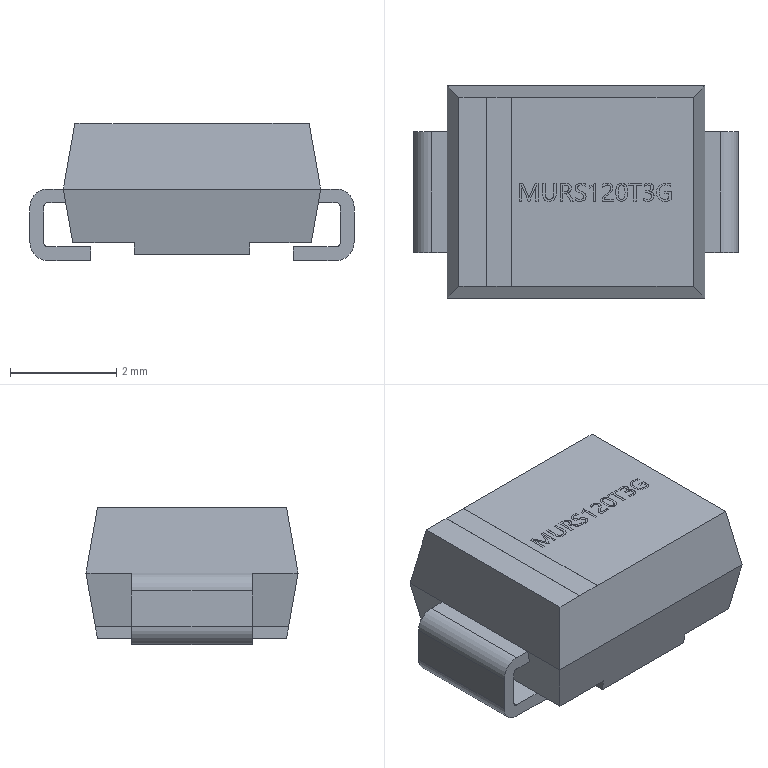Part | NX | features BREP 1 | 1 solid | 249 faces | box 6.112 x 4 x 2.584 mm | volume 44.417 mm3 | plane 161 | spline 80 | cylinder 8 | commonest cylinder face diameters 0.157 x4 0.674 x4